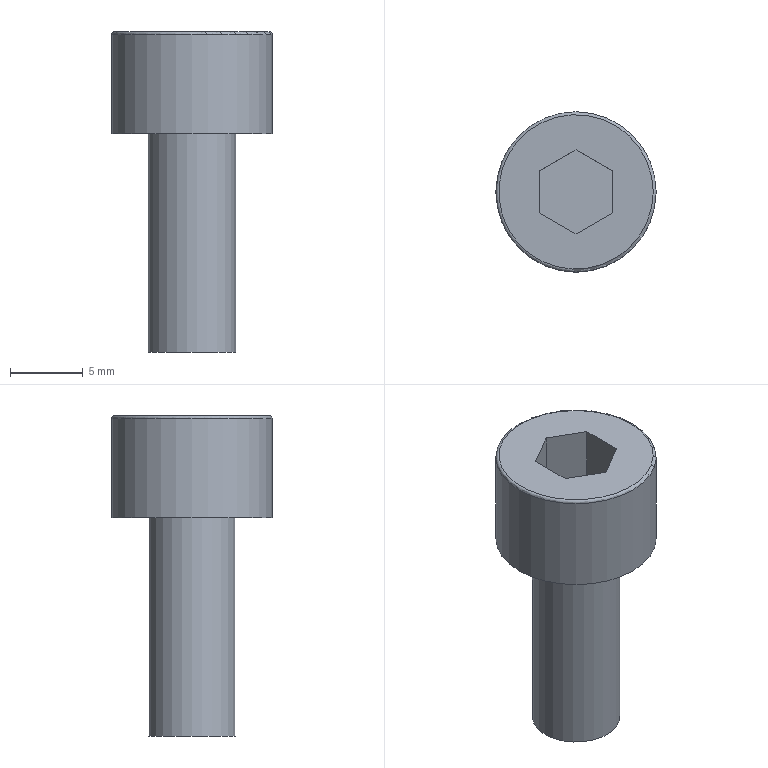Part | STEP file | solid 187 | 1 solid | 13 faces | box 11 x 11 x 22 mm | volume 1002 mm3 | plane 10 | cylinder 2 | torus 1 | commonest cylinder face diameters 6 x1 11 x1